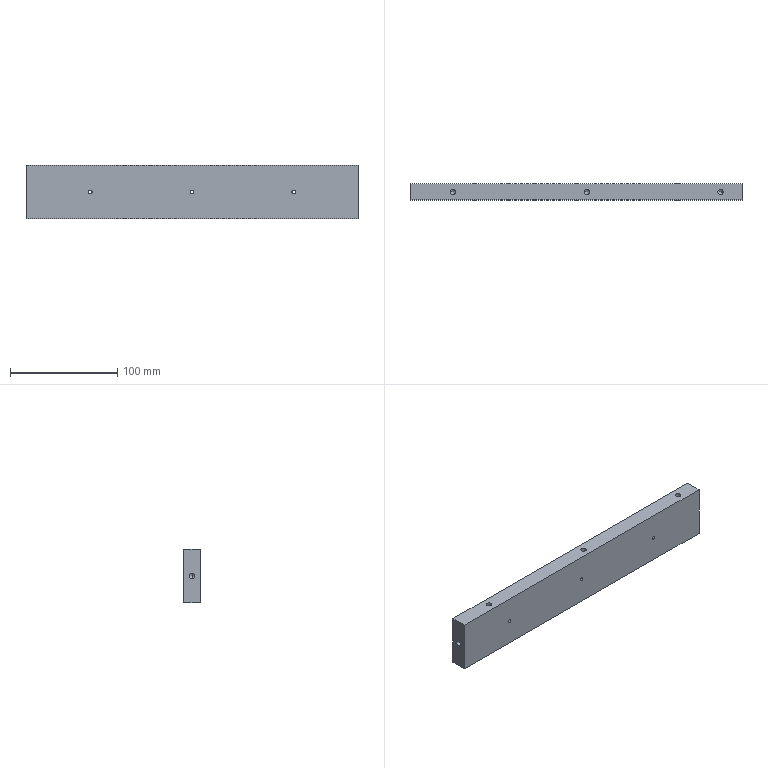Part | SolidWorks | features HoleWzd 4, Extrusion 1 | 1 solid | 32 faces | box 310 x 15 x 50 mm | volume 230397 mm3 | cylinder 16 | cone 10 | plane 6 | commonest cylinder face diameters 5 x10 3.3 x6
STEP:
#1=CARTESIAN_POINT('',(-95.,-7.5,-1.65));
#2=VERTEX_POINT('',#1);
#3=CARTESIAN_POINT('',(-95.,-7.5,1.65));
#4=VERTEX_POINT('',#3);
#5=CARTESIAN_POINT('',(-95.,-7.5,0.));
#6=DIRECTION('',(0.,1.,0.));
#7=DIRECTION('',(0.,0.,1.));
#8=AXIS2_PLACEMENT_3D('',#5,#6,#7);
#9=CIRCLE('',#8,1.65);
#10=EDGE_CURVE('',#2,#4,#9,.T.);
#11=ORIENTED_EDGE('',*,*,#10,.F.);
#12=CARTESIAN_POINT('',(-95.,7.5,-1.65));
#13=VERTEX_POINT('',#12);
#14=CARTESIAN_POINT('',(-95.,7.5,-1.65));
#15=DIRECTION('',(0.,1.,0.));
#16=VECTOR('',#15,1000.);
#17=LINE('',#14,#16);
#18=EDGE_CURVE('',#2,#13,#17,.T.);
#19=ORIENTED_EDGE('',*,*,#18,.T.);
#20=CARTESIAN_POINT('',(-95.,7.5,1.65));
#21=VERTEX_POINT('',#20);
#22=CARTESIAN_POINT('',(-95.,7.5,0.));
#23=DIRECTION('',(0.,1.,0.));
#24=DIRECTION('',(0.,0.,1.));
#25=AXIS2_PLACEMENT_3D('',#22,#23,#24);
#26=CIRCLE('',#25,1.65);
#27=EDGE_CURVE('',#13,#21,#26,.T.);
#28=ORIENTED_EDGE('',*,*,#27,.T.);
#29=CARTESIAN_POINT('',(-95.,7.5,1.65));
#30=DIRECTION('',(0.,1.,0.));
#31=VECTOR('',#30,1000.);
#32=LINE('',#29,#31);
#33=EDGE_CURVE('',#4,#21,#32,.T.);
#34=ORIENTED_EDGE('',*,*,#33,.F.);
#35=EDGE_LOOP('',(#11,#19,#28,#34));
#36=FACE_OUTER_BOUND('',#35,.T.);
#37=CARTESIAN_POINT('',(-95.,7.5,0.));
#38=DIRECTION('',(0.,1.,0.));
#39=DIRECTION('',(0.,0.,1.));
#40=AXIS2_PLACEMENT_3D('',#37,#38,#39);
#41=CYLINDRICAL_SURFACE('',#40,1.65);
#42=ADVANCED_FACE('',(#36),#41,.F.);
#43=CARTESIAN_POINT('',(0.,-7.5,-1.65));
#44=VERTEX_POINT('',#43);
#45=CARTESIAN_POINT('',(0.,-7.5,1.65));
#46=VERTEX_POINT('',#45);
#47=CARTESIAN_POINT('',(0.,-7.5,0.));
#48=DIRECTION('',(0.,1.,0.));
#49=DIRECTION('',(0.,0.,1.));
#50=AXIS2_PLACEMENT_3D('',#47,#48,#49);
#51=CIRCLE('',#50,1.65);
#52=EDGE_CURVE('',#44,#46,#51,.T.);
#53=ORIENTED_EDGE('',*,*,#52,.F.);
#54=CARTESIAN_POINT('',(0.,7.5,-1.65));
#55=VERTEX_POINT('',#54);
#56=CARTESIAN_POINT('',(0.,7.5,-1.65));
#57=DIRECTION('',(0.,1.,0.));
#58=VECTOR('',#57,1000.);
#59=LINE('',#56,#58);
#60=EDGE_CURVE('',#44,#55,#59,.T.);
#61=ORIENTED_EDGE('',*,*,#60,.T.);
#62=CARTESIAN_POINT('',(0.,7.5,1.65));
#63=VERTEX_POINT('',#62);
#64=CARTESIAN_POINT('',(0.,7.5,0.));
#65=DIRECTION('',(0.,1.,0.));
#66=DIRECTION('',(0.,0.,1.));
#67=AXIS2_PLACEMENT_3D('',#64,#65,#66);
#68=CIRCLE('',#67,1.65);
#69=EDGE_CURVE('',#55,#63,#68,.T.);
#70=ORIENTED_EDGE('',*,*,#69,.T.);
#71=CARTESIAN_POINT('',(0.,7.5,1.65));
#72=DIRECTION('',(0.,1.,0.));
#73=VECTOR('',#72,1000.);
#74=LINE('',#71,#73);
#75=EDGE_CURVE('',#46,#63,#74,.T.);
#76=ORIENTED_EDGE('',*,*,#75,.F.);
#77=EDGE_LOOP('',(#53,#61,#70,#76));
#78=FACE_OUTER_BOUND('',#77,.T.);
#79=CARTESIAN_POINT('',(0.,7.5,0.));
#80=DIRECTION('',(0.,1.,0.));
#81=DIRECTION('',(0.,0.,1.));
#82=AXIS2_PLACEMENT_3D('',#79,#80,#81);
#83=CYLINDRICAL_SURFACE('',#82,1.65);
#84=ADVANCED_FACE('',(#78),#83,.F.);
#85=CARTESIAN_POINT('',(95.,-7.5,-1.65));
#86=VERTEX_POINT('',#85);
#87=CARTESIAN_POINT('',(95.,-7.5,1.65));
#88=VERTEX_POINT('',#87);
#89=CARTESIAN_POINT('',(95.,-7.5,0.));
#90=DIRECTION('',(0.,1.,0.));
#91=DIRECTION('',(0.,0.,1.));
#92=AXIS2_PLACEMENT_3D('',#89,#90,#91);
#93=CIRCLE('',#92,1.65);
#94=EDGE_CURVE('',#86,#88,#93,.T.);
#95=ORIENTED_EDGE('',*,*,#94,.F.);
#96=CARTESIAN_POINT('',(95.,7.5,-1.65));
#97=VERTEX_POINT('',#96);
#98=CARTESIAN_POINT('',(95.,7.5,-1.65));
#99=DIRECTION('',(0.,1.,0.));
#100=VECTOR('',#99,1000.);
#101=LINE('',#98,#100);
#102=EDGE_CURVE('',#86,#97,#101,.T.);
#103=ORIENTED_EDGE('',*,*,#102,.T.);
#104=CARTESIAN_POINT('',(95.,7.5,1.65));
#105=VERTEX_POINT('',#104);
#106=CARTESIAN_POINT('',(95.,7.5,0.));
#107=DIRECTION('',(0.,1.,0.));
#108=DIRECTION('',(0.,0.,1.));
#109=AXIS2_PLACEMENT_3D('',#106,#107,#108);
#110=CIRCLE('',#109,1.65);
#111=EDGE_CURVE('',#97,#105,#110,.T.);
#112=ORIENTED_EDGE('',*,*,#111,.T.);
#113=CARTESIAN_POINT('',(95.,7.5,1.65));
#114=DIRECTION('',(0.,1.,0.));
#115=VECTOR('',#114,1000.);
#116=LINE('',#113,#115);
#117=EDGE_CURVE('',#88,#105,#116,.T.);
#118=ORIENTED_EDGE('',*,*,#117,.F.);
#119=EDGE_LOOP('',(#95,#103,#112,#118));
#120=FACE_OUTER_BOUND('',#119,.T.);
#121=CARTESIAN_POINT('',(95.,7.5,0.));
#122=DIRECTION('',(0.,1.,0.));
#123=DIRECTION('',(0.,0.,1.));
#124=AXIS2_PLACEMENT_3D('',#121,#122,#123);
#125=CYLINDRICAL_SURFACE('',#124,1.65);
#126=ADVANCED_FACE('',(#120),#125,.F.);
#127=CARTESIAN_POINT('',(-138.,0.,-2.5));
#128=VERTEX_POINT('',#127);
#129=CARTESIAN_POINT('',(-138.,0.,2.5));
#130=VERTEX_POINT('',#129);
#131=CARTESIAN_POINT('',(-138.,0.,0.));
#132=DIRECTION('',(-1.,0.,0.));
#133=DIRECTION('',(0.,0.,1.));
#134=AXIS2_PLACEMENT_3D('',#131,#132,#133);
#135=CIRCLE('',#134,2.5);
#136=EDGE_CURVE('',#128,#130,#135,.T.);
#137=ORIENTED_EDGE('',*,*,#136,.F.);
#138=CARTESIAN_POINT('',(-155.,0.,-2.5));
#139=VERTEX_POINT('',#138);
#140=CARTESIAN_POINT('',(-155.,0.,-2.5));
#141=DIRECTION('',(-1.,0.,0.));
#142=VECTOR('',#141,1000.);
#143=LINE('',#140,#142);
#144=EDGE_CURVE('',#128,#139,#143,.T.);
#145=ORIENTED_EDGE('',*,*,#144,.T.);
#146=CARTESIAN_POINT('',(-155.,0.,2.5));
#147=VERTEX_POINT('',#146);
#148=CARTESIAN_POINT('',(-155.,0.,0.));
#149=DIRECTION('',(-1.,0.,0.));
#150=DIRECTION('',(0.,0.,1.));
#151=AXIS2_PLACEMENT_3D('',#148,#149,#150);
#152=CIRCLE('',#151,2.5);
#153=EDGE_CURVE('',#139,#147,#152,.T.);
#154=ORIENTED_EDGE('',*,*,#153,.T.);
#155=CARTESIAN_POINT('',(-155.,0.,2.5));
#156=DIRECTION('',(-1.,0.,0.));
#157=VECTOR('',#156,1000.);
#158=LINE('',#155,#157);
#159=EDGE_CURVE('',#130,#147,#158,.T.);
#160=ORIENTED_EDGE('',*,*,#159,.F.);
#161=EDGE_LOOP('',(#137,#145,#154,#160));
#162=FACE_OUTER_BOUND('',#161,.T.);
#163=CARTESIAN_POINT('',(-155.,0.,0.));
#164=DIRECTION('',(-1.,0.,0.));
#165=DIRECTION('',(0.,0.,1.));
#166=AXIS2_PLACEMENT_3D('',#163,#164,#165);
#167=CYLINDRICAL_SURFACE('',#166,2.5);
#168=ADVANCED_FACE('',(#162),#167,.F.);
#169=CARTESIAN_POINT('',(-136.498,0.,0.));
#170=VERTEX_POINT('',#169);
#171=CARTESIAN_POINT('',(-138.,0.,2.5));
#172=DIRECTION('',(-0.515,0.,0.8572));
#173=VECTOR('',#172,1000.);
#174=LINE('',#171,#173);
#175=EDGE_CURVE('',#170,#130,#174,.T.);
#176=ORIENTED_EDGE('',*,*,#175,.F.);
#177=CARTESIAN_POINT('',(-138.,0.,-2.5));
#178=DIRECTION('',(-0.515,0.,-0.8572));
#179=VECTOR('',#178,1000.);
#180=LINE('',#177,#179);
#181=EDGE_CURVE('',#170,#128,#180,.T.);
#182=ORIENTED_EDGE('',*,*,#181,.T.);
#183=ORIENTED_EDGE('',*,*,#136,.T.);
#184=EDGE_LOOP('',(#176,#182,#183));
#185=FACE_OUTER_BOUND('',#184,.T.);
#186=CARTESIAN_POINT('',(-138.,0.,0.));
#187=DIRECTION('',(-1.,0.,0.));
#188=DIRECTION('',(0.,0.,1.));
#189=AXIS2_PLACEMENT_3D('',#186,#187,#188);
#190=CONICAL_SURFACE('',#189,2.5,1.03);
#191=ADVANCED_FACE('',(#185),#190,.F.);
#192=CARTESIAN_POINT('',(138.,0.,2.5));
#193=VERTEX_POINT('',#192);
#194=CARTESIAN_POINT('',(138.,0.,-2.5));
#195=VERTEX_POINT('',#194);
#196=CARTESIAN_POINT('',(138.,0.,0.));
#197=DIRECTION('',(1.,0.,0.));
#198=DIRECTION('',(0.,0.,-1.));
#199=AXIS2_PLACEMENT_3D('',#196,#197,#198);
#200=CIRCLE('',#199,2.5);
#201=EDGE_CURVE('',#193,#195,#200,.T.);
#202=ORIENTED_EDGE('',*,*,#201,.F.);
#203=CARTESIAN_POINT('',(155.,0.,2.5));
#204=VERTEX_POINT('',#203);
#205=CARTESIAN_POINT('',(155.,0.,2.5));
#206=DIRECTION('',(1.,0.,0.));
#207=VECTOR('',#206,1000.);
#208=LINE('',#205,#207);
#209=EDGE_CURVE('',#193,#204,#208,.T.);
#210=ORIENTED_EDGE('',*,*,#209,.T.);
#211=CARTESIAN_POINT('',(155.,0.,-2.5));
#212=VERTEX_POINT('',#211);
#213=CARTESIAN_POINT('',(155.,0.,0.));
#214=DIRECTION('',(1.,0.,0.));
#215=DIRECTION('',(0.,0.,-1.));
#216=AXIS2_PLACEMENT_3D('',#213,#214,#215);
#217=CIRCLE('',#216,2.5);
#218=EDGE_CURVE('',#204,#212,#217,.T.);
#219=ORIENTED_EDGE('',*,*,#218,.T.);
#220=CARTESIAN_POINT('',(155.,0.,-2.5));
#221=DIRECTION('',(1.,0.,0.));
#222=VECTOR('',#221,1000.);
#223=LINE('',#220,#222);
#224=EDGE_CURVE('',#195,#212,#223,.T.);
#225=ORIENTED_EDGE('',*,*,#224,.F.);
#226=EDGE_LOOP('',(#202,#210,#219,#225));
#227=FACE_OUTER_BOUND('',#226,.T.);
#228=CARTESIAN_POINT('',(155.,0.,0.));
#229=DIRECTION('',(1.,0.,0.));
#230=DIRECTION('',(0.,0.,-1.));
#231=AXIS2_PLACEMENT_3D('',#228,#229,#230);
#232=CYLINDRICAL_SURFACE('',#231,2.5);
#233=ADVANCED_FACE('',(#227),#232,.F.);
#234=CARTESIAN_POINT('',(136.498,0.,0.));
#235=VERTEX_POINT('',#234);
#236=CARTESIAN_POINT('',(138.,0.,-2.5));
#237=DIRECTION('',(0.515,0.,-0.8572));
#238=VECTOR('',#237,1000.);
#239=LINE('',#236,#238);
#240=EDGE_CURVE('',#235,#195,#239,.T.);
#241=ORIENTED_EDGE('',*,*,#240,.F.);
#242=CARTESIAN_POINT('',(138.,0.,2.5));
#243=DIRECTION('',(0.515,0.,0.8572));
#244=VECTOR('',#243,1000.);
#245=LINE('',#242,#244);
#246=EDGE_CURVE('',#235,#193,#245,.T.);
#247=ORIENTED_EDGE('',*,*,#246,.T.);
#248=ORIENTED_EDGE('',*,*,#201,.T.);
#249=EDGE_LOOP('',(#241,#247,#248));
#250=FACE_OUTER_BOUND('',#249,.T.);
#251=CARTESIAN_POINT('',(138.,0.,0.));
#252=DIRECTION('',(1.,0.,0.));
#253=DIRECTION('',(0.,0.,-1.));
#254=AXIS2_PLACEMENT_3D('',#251,#252,#253);
#255=CONICAL_SURFACE('',#254,2.5,1.03);
#256=ADVANCED_FACE('',(#250),#255,.F.);
#257=CARTESIAN_POINT('',(-117.5,0.,8.));
#258=VERTEX_POINT('',#257);
#259=CARTESIAN_POINT('',(-112.5,0.,8.));
#260=VERTEX_POINT('',#259);
#261=CARTESIAN_POINT('',(-115.,0.,8.));
#262=DIRECTION('',(0.,0.,1.));
#263=DIRECTION('',(1.,0.,0.));
#264=AXIS2_PLACEMENT_3D('',#261,#262,#263);
#265=CIRCLE('',#264,2.5);
#266=EDGE_CURVE('',#258,#260,#265,.T.);
#267=ORIENTED_EDGE('',*,*,#266,.F.);
#268=CARTESIAN_POINT('',(-117.5,0.,25.));
#269=VERTEX_POINT('',#268);
#270=CARTESIAN_POINT('',(-117.5,0.,25.));
#271=DIRECTION('',(0.,0.,1.));
#272=VECTOR('',#271,1000.);
#273=LINE('',#270,#272);
#274=EDGE_CURVE('',#258,#269,#273,.T.);
#275=ORIENTED_EDGE('',*,*,#274,.T.);
#276=CARTESIAN_POINT('',(-112.5,0.,25.));
#277=VERTEX_POINT('',#276);
#278=CARTESIAN_POINT('',(-115.,0.,25.));
#279=DIRECTION('',(0.,0.,1.));
#280=DIRECTION('',(1.,0.,0.));
#281=AXIS2_PLACEMENT_3D('',#278,#279,#280);
#282=CIRCLE('',#281,2.5);
#283=EDGE_CURVE('',#269,#277,#282,.T.);
#284=ORIENTED_EDGE('',*,*,#283,.T.);
#285=CARTESIAN_POINT('',(-112.5,0.,25.));
#286=DIRECTION('',(0.,0.,1.));
#287=VECTOR('',#286,1000.);
#288=LINE('',#285,#287);
#289=EDGE_CURVE('',#260,#277,#288,.T.);
#290=ORIENTED_EDGE('',*,*,#289,.F.);
#291=EDGE_LOOP('',(#267,#275,#284,#290));
#292=FACE_OUTER_BOUND('',#291,.T.);
#293=CARTESIAN_POINT('',(-115.,0.,25.));
#294=DIRECTION('',(0.,0.,1.));
#295=DIRECTION('',(1.,0.,0.));
#296=AXIS2_PLACEMENT_3D('',#293,#294,#295);
#297=CYLINDRICAL_SURFACE('',#296,2.5);
#298=ADVANCED_FACE('',(#292),#297,.F.);
#299=CARTESIAN_POINT('',(-115.,0.,6.498));
#300=VERTEX_POINT('',#299);
#301=CARTESIAN_POINT('',(-112.5,0.,8.));
#302=DIRECTION('',(0.8572,0.,0.515));
#303=VECTOR('',#302,1000.);
#304=LINE('',#301,#303);
#305=EDGE_CURVE('',#300,#260,#304,.T.);
#306=ORIENTED_EDGE('',*,*,#305,.F.);
#307=CARTESIAN_POINT('',(-117.5,0.,8.));
#308=DIRECTION('',(-0.8572,0.,0.515));
#309=VECTOR('',#308,1000.);
#310=LINE('',#307,#309);
#311=EDGE_CURVE('',#300,#258,#310,.T.);
#312=ORIENTED_EDGE('',*,*,#311,.T.);
#313=ORIENTED_EDGE('',*,*,#266,.T.);
#314=EDGE_LOOP('',(#306,#312,#313));
#315=FACE_OUTER_BOUND('',#314,.T.);
#316=CARTESIAN_POINT('',(-115.,0.,8.));
#317=DIRECTION('',(0.,0.,1.));
#318=DIRECTION('',(1.,0.,0.));
#319=AXIS2_PLACEMENT_3D('',#316,#317,#318);
#320=CONICAL_SURFACE('',#319,2.5,1.03);
#321=ADVANCED_FACE('',(#315),#320,.F.);
#322=CARTESIAN_POINT('',(7.5,0.,8.));
#323=VERTEX_POINT('',#322);
#324=CARTESIAN_POINT('',(12.5,0.,8.));
#325=VERTEX_POINT('',#324);
#326=CARTESIAN_POINT('',(10.,0.,8.));
#327=DIRECTION('',(0.,0.,1.));
#328=DIRECTION('',(1.,0.,0.));
#329=AXIS2_PLACEMENT_3D('',#326,#327,#328);
#330=CIRCLE('',#329,2.5);
#331=EDGE_CURVE('',#323,#325,#330,.T.);
#332=ORIENTED_EDGE('',*,*,#331,.F.);
#333=CARTESIAN_POINT('',(7.5,0.,25.));
#334=VERTEX_POINT('',#333);
#335=CARTESIAN_POINT('',(7.5,0.,25.));
#336=DIRECTION('',(0.,0.,1.));
#337=VECTOR('',#336,1000.);
#338=LINE('',#335,#337);
#339=EDGE_CURVE('',#323,#334,#338,.T.);
#340=ORIENTED_EDGE('',*,*,#339,.T.);
#341=CARTESIAN_POINT('',(12.5,0.,25.));
#342=VERTEX_POINT('',#341);
#343=CARTESIAN_POINT('',(10.,0.,25.));
#344=DIRECTION('',(0.,0.,1.));
#345=DIRECTION('',(1.,0.,0.));
#346=AXIS2_PLACEMENT_3D('',#343,#344,#345);
#347=CIRCLE('',#346,2.5);
#348=EDGE_CURVE('',#334,#342,#347,.T.);
#349=ORIENTED_EDGE('',*,*,#348,.T.);
#350=CARTESIAN_POINT('',(12.5,0.,25.));
#351=DIRECTION('',(0.,0.,1.));
#352=VECTOR('',#351,1000.);
#353=LINE('',#350,#352);
#354=EDGE_CURVE('',#325,#342,#353,.T.);
#355=ORIENTED_EDGE('',*,*,#354,.F.);
#356=EDGE_LOOP('',(#332,#340,#349,#355));
#357=FACE_OUTER_BOUND('',#356,.T.);
#358=CARTESIAN_POINT('',(10.,0.,25.));
#359=DIRECTION('',(0.,0.,1.));
#360=DIRECTION('',(1.,0.,0.));
#361=AXIS2_PLACEMENT_3D('',#358,#359,#360);
#362=CYLINDRICAL_SURFACE('',#361,2.5);
#363=ADVANCED_FACE('',(#357),#362,.F.);
#364=CARTESIAN_POINT('',(10.,0.,6.498));
#365=VERTEX_POINT('',#364);
#366=CARTESIAN_POINT('',(12.5,0.,8.));
#367=DIRECTION('',(0.8572,0.,0.515));
#368=VECTOR('',#367,1000.);
#369=LINE('',#366,#368);
#370=EDGE_CURVE('',#365,#325,#369,.T.);
#371=ORIENTED_EDGE('',*,*,#370,.F.);
#372=CARTESIAN_POINT('',(7.5,0.,8.));
#373=DIRECTION('',(-0.8572,0.,0.515));
#374=VECTOR('',#373,1000.);
#375=LINE('',#372,#374);
#376=EDGE_CURVE('',#365,#323,#375,.T.);
#377=ORIENTED_EDGE('',*,*,#376,.T.);
#378=ORIENTED_EDGE('',*,*,#331,.T.);
#379=EDGE_LOOP('',(#371,#377,#378));
#380=FACE_OUTER_BOUND('',#379,.T.);
#381=CARTESIAN_POINT('',(10.,0.,8.));
#382=DIRECTION('',(0.,0.,1.));
#383=DIRECTION('',(1.,0.,0.));
#384=AXIS2_PLACEMENT_3D('',#381,#382,#383);
#385=CONICAL_SURFACE('',#384,2.5,1.03);
#386=ADVANCED_FACE('',(#380),#385,.F.);
#387=CARTESIAN_POINT('',(132.5,0.,8.));
#388=VERTEX_POINT('',#387);
#389=CARTESIAN_POINT('',(137.5,0.,8.));
#390=VERTEX_POINT('',#389);
#391=CARTESIAN_POINT('',(135.,0.,8.));
#392=DIRECTION('',(0.,0.,1.));
#393=DIRECTION('',(1.,0.,0.));
#394=AXIS2_PLACEMENT_3D('',#391,#392,#393);
#395=CIRCLE('',#394,2.5);
#396=EDGE_CURVE('',#388,#390,#395,.T.);
#397=ORIENTED_EDGE('',*,*,#396,.F.);
#398=CARTESIAN_POINT('',(132.5,0.,25.));
#399=VERTEX_POINT('',#398);
#400=CARTESIAN_POINT('',(132.5,0.,25.));
#401=DIRECTION('',(0.,0.,1.));
#402=VECTOR('',#401,1000.);
#403=LINE('',#400,#402);
#404=EDGE_CURVE('',#388,#399,#403,.T.);
#405=ORIENTED_EDGE('',*,*,#404,.T.);
#406=CARTESIAN_POINT('',(137.5,0.,25.));
#407=VERTEX_POINT('',#406);
#408=CARTESIAN_POINT('',(135.,0.,25.));
#409=DIRECTION('',(0.,0.,1.));
#410=DIRECTION('',(1.,0.,0.));
#411=AXIS2_PLACEMENT_3D('',#408,#409,#410);
#412=CIRCLE('',#411,2.5);
#413=EDGE_CURVE('',#399,#407,#412,.T.);
#414=ORIENTED_EDGE('',*,*,#413,.T.);
#415=CARTESIAN_POINT('',(137.5,0.,25.));
#416=DIRECTION('',(0.,0.,1.));
#417=VECTOR('',#416,1000.);
#418=LINE('',#415,#417);
#419=EDGE_CURVE('',#390,#407,#418,.T.);
#420=ORIENTED_EDGE('',*,*,#419,.F.);
#421=EDGE_LOOP('',(#397,#405,#414,#420));
#422=FACE_OUTER_BOUND('',#421,.T.);
#423=CARTESIAN_POINT('',(135.,0.,25.));
#424=DIRECTION('',(0.,0.,1.));
#425=DIRECTION('',(1.,0.,0.));
#426=AXIS2_PLACEMENT_3D('',#423,#424,#425);
#427=CYLINDRICAL_SURFACE('',#426,2.5);
#428=ADVANCED_FACE('',(#422),#427,.F.);
#429=CARTESIAN_POINT('',(135.,0.,6.498));
#430=VERTEX_POINT('',#429);
#431=CARTESIAN_POINT('',(137.5,0.,8.));
#432=DIRECTION('',(0.8572,0.,0.515));
#433=VECTOR('',#432,1000.);
#434=LINE('',#431,#433);
#435=EDGE_CURVE('',#430,#390,#434,.T.);
#436=ORIENTED_EDGE('',*,*,#435,.F.);
#437=CARTESIAN_POINT('',(132.5,0.,8.));
#438=DIRECTION('',(-0.8572,0.,0.515));
#439=VECTOR('',#438,1000.);
#440=LINE('',#437,#439);
#441=EDGE_CURVE('',#430,#388,#440,.T.);
#442=ORIENTED_EDGE('',*,*,#441,.T.);
#443=ORIENTED_EDGE('',*,*,#396,.T.);
#444=EDGE_LOOP('',(#436,#442,#443));
#445=FACE_OUTER_BOUND('',#444,.T.);
#446=CARTESIAN_POINT('',(135.,0.,8.));
#447=DIRECTION('',(0.,0.,1.));
#448=DIRECTION('',(1.,0.,0.));
#449=AXIS2_PLACEMENT_3D('',#446,#447,#448);
#450=CONICAL_SURFACE('',#449,2.5,1.03);
#451=ADVANCED_FACE('',(#445),#450,.F.);
#452=CARTESIAN_POINT('',(-155.,0.,0.));
#453=DIRECTION('',(-1.,0.,0.));
#454=DIRECTION('',(0.,0.,1.));
#455=AXIS2_PLACEMENT_3D('',#452,#453,#454);
#456=CIRCLE('',#455,2.5);
#457=EDGE_CURVE('',#147,#139,#456,.T.);
#458=ORIENTED_EDGE('',*,*,#457,.F.);
#459=ORIENTED_EDGE('',*,*,#153,.F.);
#460=EDGE_LOOP('',(#458,#459));
#461=FACE_BOUND('',#460,.T.);
#462=CARTESIAN_POINT('',(-155.,-7.5,-25.));
#463=VERTEX_POINT('',#462);
#464=CARTESIAN_POINT('',(-155.,-7.5,25.));
#465=VERTEX_POINT('',#464);
#466=CARTESIAN_POINT('',(-155.,-7.5,25.));
#467=DIRECTION('',(0.,0.,1.));
#468=VECTOR('',#467,1000.);
#469=LINE('',#466,#468);
#470=EDGE_CURVE('',#463,#465,#469,.T.);
#471=ORIENTED_EDGE('',*,*,#470,.T.);
#472=CARTESIAN_POINT('',(-155.,7.5,25.));
#473=VERTEX_POINT('',#472);
#474=CARTESIAN_POINT('',(-155.,7.5,25.));
#475=DIRECTION('',(0.,-1.,0.));
#476=VECTOR('',#475,1000.);
#477=LINE('',#474,#476);
#478=EDGE_CURVE('',#473,#465,#477,.T.);
#479=ORIENTED_EDGE('',*,*,#478,.F.);
#480=CARTESIAN_POINT('',(-155.,7.5,-25.));
#481=VERTEX_POINT('',#480);
#482=CARTESIAN_POINT('',(-155.,7.5,25.));
#483=DIRECTION('',(0.,0.,1.));
#484=VECTOR('',#483,1000.);
#485=LINE('',#482,#484);
#486=EDGE_CURVE('',#481,#473,#485,.T.);
#487=ORIENTED_EDGE('',*,*,#486,.F.);
#488=CARTESIAN_POINT('',(-155.,7.5,-25.));
#489=DIRECTION('',(0.,-1.,0.));
#490=VECTOR('',#489,1000.);
#491=LINE('',#488,#490);
#492=EDGE_CURVE('',#481,#463,#491,.T.);
#493=ORIENTED_EDGE('',*,*,#492,.T.);
#494=EDGE_LOOP('',(#471,#479,#487,#493));
#495=FACE_OUTER_BOUND('',#494,.T.);
#496=CARTESIAN_POINT('',(-155.,7.5,25.));
#497=DIRECTION('',(1.,0.,0.));
#498=DIRECTION('',(0.,0.,-1.));
#499=AXIS2_PLACEMENT_3D('',#496,#497,#498);
#500=PLANE('',#499);
#501=ADVANCED_FACE('',(#461,#495),#500,.F.);
#502=CARTESIAN_POINT('',(-115.,0.,25.));
#503=DIRECTION('',(0.,0.,1.));
#504=DIRECTION('',(1.,0.,0.));
#505=AXIS2_PLACEMENT_3D('',#502,#503,#504);
#506=CIRCLE('',#505,2.5);
#507=EDGE_CURVE('',#277,#269,#506,.T.);
#508=ORIENTED_EDGE('',*,*,#507,.F.);
#509=ORIENTED_EDGE('',*,*,#283,.F.);
#510=EDGE_LOOP('',(#508,#509));
#511=FACE_BOUND('',#510,.T.);
#512=CARTESIAN_POINT('',(10.,0.,25.));
#513=DIRECTION('',(0.,0.,1.));
#514=DIRECTION('',(1.,0.,0.));
#515=AXIS2_PLACEMENT_3D('',#512,#513,#514);
#516=CIRCLE('',#515,2.5);
#517=EDGE_CURVE('',#342,#334,#516,.T.);
#518=ORIENTED_EDGE('',*,*,#517,.F.);
#519=ORIENTED_EDGE('',*,*,#348,.F.);
#520=EDGE_LOOP('',(#518,#519));
#521=FACE_BOUND('',#520,.T.);
#522=CARTESIAN_POINT('',(135.,0.,25.));
#523=DIRECTION('',(0.,0.,1.));
#524=DIRECTION('',(1.,0.,0.));
#525=AXIS2_PLACEMENT_3D('',#522,#523,#524);
#526=CIRCLE('',#525,2.5);
#527=EDGE_CURVE('',#407,#399,#526,.T.);
#528=ORIENTED_EDGE('',*,*,#527,.F.);
#529=ORIENTED_EDGE('',*,*,#413,.F.);
#530=EDGE_LOOP('',(#528,#529));
#531=FACE_BOUND('',#530,.T.);
#532=CARTESIAN_POINT('',(155.,-7.5,25.));
#533=VERTEX_POINT('',#532);
#534=CARTESIAN_POINT('',(155.,-7.5,25.));
#535=DIRECTION('',(1.,0.,0.));
#536=VECTOR('',#535,1000.);
#537=LINE('',#534,#536);
#538=EDGE_CURVE('',#465,#533,#537,.T.);
#539=ORIENTED_EDGE('',*,*,#538,.T.);
#540=CARTESIAN_POINT('',(155.,7.5,25.));
#541=VERTEX_POINT('',#540);
#542=CARTESIAN_POINT('',(155.,7.5,25.));
#543=DIRECTION('',(0.,-1.,0.));
#544=VECTOR('',#543,1000.);
#545=LINE('',#542,#544);
#546=EDGE_CURVE('',#541,#533,#545,.T.);
#547=ORIENTED_EDGE('',*,*,#546,.F.);
#548=CARTESIAN_POINT('',(155.,7.5,25.));
#549=DIRECTION('',(1.,0.,0.));
#550=VECTOR('',#549,1000.);
#551=LINE('',#548,#550);
#552=EDGE_CURVE('',#473,#541,#551,.T.);
#553=ORIENTED_EDGE('',*,*,#552,.F.);
#554=ORIENTED_EDGE('',*,*,#478,.T.);
#555=EDGE_LOOP('',(#539,#547,#553,#554));
#556=FACE_OUTER_BOUND('',#555,.T.);
#557=CARTESIAN_POINT('',(155.,7.5,25.));
#558=DIRECTION('',(0.,0.,-1.));
#559=DIRECTION('',(-1.,0.,0.));
#560=AXIS2_PLACEMENT_3D('',#557,#558,#559);
#561=PLANE('',#560);
#562=ADVANCED_FACE('',(#511,#521,#531,#556),#561,.F.);
#563=CARTESIAN_POINT('',(155.,0.,0.));
#564=DIRECTION('',(1.,0.,0.));
#565=DIRECTION('',(0.,0.,-1.));
#566=AXIS2_PLACEMENT_3D('',#563,#564,#565);
#567=CIRCLE('',#566,2.5);
#568=EDGE_CURVE('',#212,#204,#567,.T.);
#569=ORIENTED_EDGE('',*,*,#568,.F.);
#570=ORIENTED_EDGE('',*,*,#218,.F.);
#571=EDGE_LOOP('',(#569,#570));
#572=FACE_BOUND('',#571,.T.);
#573=CARTESIAN_POINT('',(155.,-7.5,-25.));
#574=VERTEX_POINT('',#573);
#575=CARTESIAN_POINT('',(155.,-7.5,25.));
#576=DIRECTION('',(0.,0.,-1.));
#577=VECTOR('',#576,1000.);
#578=LINE('',#575,#577);
#579=EDGE_CURVE('',#533,#574,#578,.T.);
#580=ORIENTED_EDGE('',*,*,#579,.T.);
#581=CARTESIAN_POINT('',(155.,7.5,-25.));
#582=VERTEX_POINT('',#581);
#583=CARTESIAN_POINT('',(155.,7.5,-25.));
#584=DIRECTION('',(0.,-1.,0.));
#585=VECTOR('',#584,1000.);
#586=LINE('',#583,#585);
#587=EDGE_CURVE('',#582,#574,#586,.T.);
#588=ORIENTED_EDGE('',*,*,#587,.F.);
#589=CARTESIAN_POINT('',(155.,7.5,25.));
#590=DIRECTION('',(0.,0.,-1.));
#591=VECTOR('',#590,1000.);
#592=LINE('',#589,#591);
#593=EDGE_CURVE('',#541,#582,#592,.T.);
#594=ORIENTED_EDGE('',*,*,#593,.F.);
#595=ORIENTED_EDGE('',*,*,#546,.T.);
#596=EDGE_LOOP('',(#580,#588,#594,#595));
#597=FACE_OUTER_BOUND('',#596,.T.);
#598=CARTESIAN_POINT('',(155.,7.5,25.));
#599=DIRECTION('',(-1.,0.,0.));
#600=DIRECTION('',(0.,0.,1.));
#601=AXIS2_PLACEMENT_3D('',#598,#599,#600);
#602=PLANE('',#601);
#603=ADVANCED_FACE('',(#572,#597),#602,.F.);
#604=CARTESIAN_POINT('',(155.,-7.5,-25.));
#605=DIRECTION('',(-1.,0.,0.));
#606=VECTOR('',#605,1000.);
#607=LINE('',#604,#606);
#608=EDGE_CURVE('',#574,#463,#607,.T.);
#609=ORIENTED_EDGE('',*,*,#608,.T.);
#610=ORIENTED_EDGE('',*,*,#492,.F.);
#611=CARTESIAN_POINT('',(155.,7.5,-25.));
#612=DIRECTION('',(-1.,0.,0.));
#613=VECTOR('',#612,1000.);
#614=LINE('',#611,#613);
#615=EDGE_CURVE('',#582,#481,#614,.T.);
#616=ORIENTED_EDGE('',*,*,#615,.F.);
#617=ORIENTED_EDGE('',*,*,#587,.T.);
#618=EDGE_LOOP('',(#609,#610,#616,#617));
#619=FACE_OUTER_BOUND('',#618,.T.);
#620=CARTESIAN_POINT('',(155.,7.5,-25.));
#621=DIRECTION('',(0.,0.,1.));
#622=DIRECTION('',(1.,0.,0.));
#623=AXIS2_PLACEMENT_3D('',#620,#621,#622);
#624=PLANE('',#623);
#625=ADVANCED_FACE('',(#619),#624,.F.);
#626=CARTESIAN_POINT('',(-95.,7.5,0.));
#627=DIRECTION('',(0.,1.,0.));
#628=DIRECTION('',(0.,0.,1.));
#629=AXIS2_PLACEMENT_3D('',#626,#627,#628);
#630=CIRCLE('',#629,1.65);
#631=EDGE_CURVE('',#21,#13,#630,.T.);
#632=ORIENTED_EDGE('',*,*,#631,.F.);
#633=ORIENTED_EDGE('',*,*,#27,.F.);
#634=EDGE_LOOP('',(#632,#633));
#635=FACE_BOUND('',#634,.T.);
#636=CARTESIAN_POINT('',(0.,7.5,0.));
#637=DIRECTION('',(0.,1.,0.));
#638=DIRECTION('',(0.,0.,1.));
#639=AXIS2_PLACEMENT_3D('',#636,#637,#638);
#640=CIRCLE('',#639,1.65);
#641=EDGE_CURVE('',#63,#55,#640,.T.);
#642=ORIENTED_EDGE('',*,*,#641,.F.);
#643=ORIENTED_EDGE('',*,*,#69,.F.);
#644=EDGE_LOOP('',(#642,#643));
#645=FACE_BOUND('',#644,.T.);
#646=CARTESIAN_POINT('',(95.,7.5,0.));
#647=DIRECTION('',(0.,1.,0.));
#648=DIRECTION('',(0.,0.,1.));
#649=AXIS2_PLACEMENT_3D('',#646,#647,#648);
#650=CIRCLE('',#649,1.65);
#651=EDGE_CURVE('',#105,#97,#650,.T.);
#652=ORIENTED_EDGE('',*,*,#651,.F.);
#653=ORIENTED_EDGE('',*,*,#111,.F.);
#654=EDGE_LOOP('',(#652,#653));
#655=FACE_BOUND('',#654,.T.);
#656=ORIENTED_EDGE('',*,*,#486,.T.);
#657=ORIENTED_EDGE('',*,*,#552,.T.);
#658=ORIENTED_EDGE('',*,*,#593,.T.);
#659=ORIENTED_EDGE('',*,*,#615,.T.);
#660=EDGE_LOOP('',(#656,#657,#658,#659));
#661=FACE_OUTER_BOUND('',#660,.T.);
#662=CARTESIAN_POINT('',(0.,7.5,0.));
#663=DIRECTION('',(0.,1.,0.));
#664=DIRECTION('',(0.,0.,1.));
#665=AXIS2_PLACEMENT_3D('',#662,#663,#664);
#666=PLANE('',#665);
#667=ADVANCED_FACE('',(#635,#645,#655,#661),#666,.T.);
#668=CARTESIAN_POINT('',(-95.,-7.5,0.));
#669=DIRECTION('',(0.,1.,0.));
#670=DIRECTION('',(0.,0.,1.));
#671=AXIS2_PLACEMENT_3D('',#668,#669,#670);
#672=CIRCLE('',#671,1.65);
#673=EDGE_CURVE('',#4,#2,#672,.T.);
#674=ORIENTED_EDGE('',*,*,#673,.T.);
#675=ORIENTED_EDGE('',*,*,#10,.T.);
#676=EDGE_LOOP('',(#674,#675));
#677=FACE_BOUND('',#676,.T.);
#678=CARTESIAN_POINT('',(0.,-7.5,0.));
#679=DIRECTION('',(0.,1.,0.));
#680=DIRECTION('',(0.,0.,1.));
#681=AXIS2_PLACEMENT_3D('',#678,#679,#680);
#682=CIRCLE('',#681,1.65);
#683=EDGE_CURVE('',#46,#44,#682,.T.);
#684=ORIENTED_EDGE('',*,*,#683,.T.);
#685=ORIENTED_EDGE('',*,*,#52,.T.);
#686=EDGE_LOOP('',(#684,#685));
#687=FACE_BOUND('',#686,.T.);
#688=CARTESIAN_POINT('',(95.,-7.5,0.));
#689=DIRECTION('',(0.,1.,0.));
#690=DIRECTION('',(0.,0.,1.));
#691=AXIS2_PLACEMENT_3D('',#688,#689,#690);
#692=CIRCLE('',#691,1.65);
#693=EDGE_CURVE('',#88,#86,#692,.T.);
#694=ORIENTED_EDGE('',*,*,#693,.T.);
#695=ORIENTED_EDGE('',*,*,#94,.T.);
#696=EDGE_LOOP('',(#694,#695));
#697=FACE_BOUND('',#696,.T.);
#698=ORIENTED_EDGE('',*,*,#470,.F.);
#699=ORIENTED_EDGE('',*,*,#608,.F.);
#700=ORIENTED_EDGE('',*,*,#579,.F.);
#701=ORIENTED_EDGE('',*,*,#538,.F.);
#702=EDGE_LOOP('',(#698,#699,#700,#701));
#703=FACE_OUTER_BOUND('',#702,.T.);
#704=CARTESIAN_POINT('',(0.,-7.5,0.));
#705=DIRECTION('',(0.,1.,0.));
#706=DIRECTION('',(0.,0.,1.));
#707=AXIS2_PLACEMENT_3D('',#704,#705,#706);
#708=PLANE('',#707);
#709=ADVANCED_FACE('',(#677,#687,#697,#703),#708,.F.);
#710=ORIENTED_EDGE('',*,*,#441,.F.);
#711=ORIENTED_EDGE('',*,*,#435,.T.);
#712=CARTESIAN_POINT('',(135.,0.,8.));
#713=DIRECTION('',(0.,0.,1.));
#714=DIRECTION('',(1.,0.,0.));
#715=AXIS2_PLACEMENT_3D('',#712,#713,#714);
#716=CIRCLE('',#715,2.5);
#717=EDGE_CURVE('',#390,#388,#716,.T.);
#718=ORIENTED_EDGE('',*,*,#717,.T.);
#719=EDGE_LOOP('',(#710,#711,#718));
#720=FACE_OUTER_BOUND('',#719,.T.);
#721=CARTESIAN_POINT('',(135.,0.,8.));
#722=DIRECTION('',(0.,0.,1.));
#723=DIRECTION('',(1.,0.,0.));
#724=AXIS2_PLACEMENT_3D('',#721,#722,#723);
#725=CONICAL_SURFACE('',#724,2.5,1.03);
#726=ADVANCED_FACE('',(#720),#725,.F.);
#727=ORIENTED_EDGE('',*,*,#404,.F.);
#728=ORIENTED_EDGE('',*,*,#717,.F.);
#729=ORIENTED_EDGE('',*,*,#419,.T.);
#730=ORIENTED_EDGE('',*,*,#527,.T.);
#731=EDGE_LOOP('',(#727,#728,#729,#730));
#732=FACE_OUTER_BOUND('',#731,.T.);
#733=CARTESIAN_POINT('',(135.,0.,25.));
#734=DIRECTION('',(0.,0.,1.));
#735=DIRECTION('',(1.,0.,0.));
#736=AXIS2_PLACEMENT_3D('',#733,#734,#735);
#737=CYLINDRICAL_SURFACE('',#736,2.5);
#738=ADVANCED_FACE('',(#732),#737,.F.);
#739=ORIENTED_EDGE('',*,*,#376,.F.);
#740=ORIENTED_EDGE('',*,*,#370,.T.);
#741=CARTESIAN_POINT('',(10.,0.,8.));
#742=DIRECTION('',(0.,0.,1.));
#743=DIRECTION('',(1.,0.,0.));
#744=AXIS2_PLACEMENT_3D('',#741,#742,#743);
#745=CIRCLE('',#744,2.5);
#746=EDGE_CURVE('',#325,#323,#745,.T.);
#747=ORIENTED_EDGE('',*,*,#746,.T.);
#748=EDGE_LOOP('',(#739,#740,#747));
#749=FACE_OUTER_BOUND('',#748,.T.);
#750=CARTESIAN_POINT('',(10.,0.,8.));
#751=DIRECTION('',(0.,0.,1.));
#752=DIRECTION('',(1.,0.,0.));
#753=AXIS2_PLACEMENT_3D('',#750,#751,#752);
#754=CONICAL_SURFACE('',#753,2.5,1.03);
#755=ADVANCED_FACE('',(#749),#754,.F.);
#756=ORIENTED_EDGE('',*,*,#339,.F.);
#757=ORIENTED_EDGE('',*,*,#746,.F.);
#758=ORIENTED_EDGE('',*,*,#354,.T.);
#759=ORIENTED_EDGE('',*,*,#517,.T.);
#760=EDGE_LOOP('',(#756,#757,#758,#759));
#761=FACE_OUTER_BOUND('',#760,.T.);
#762=CARTESIAN_POINT('',(10.,0.,25.));
#763=DIRECTION('',(0.,0.,1.));
#764=DIRECTION('',(1.,0.,0.));
#765=AXIS2_PLACEMENT_3D('',#762,#763,#764);
#766=CYLINDRICAL_SURFACE('',#765,2.5);
#767=ADVANCED_FACE('',(#761),#766,.F.);
#768=ORIENTED_EDGE('',*,*,#311,.F.);
#769=ORIENTED_EDGE('',*,*,#305,.T.);
#770=CARTESIAN_POINT('',(-115.,0.,8.));
#771=DIRECTION('',(0.,0.,1.));
#772=DIRECTION('',(1.,0.,0.));
#773=AXIS2_PLACEMENT_3D('',#770,#771,#772);
#774=CIRCLE('',#773,2.5);
#775=EDGE_CURVE('',#260,#258,#774,.T.);
#776=ORIENTED_EDGE('',*,*,#775,.T.);
#777=EDGE_LOOP('',(#768,#769,#776));
#778=FACE_OUTER_BOUND('',#777,.T.);
#779=CARTESIAN_POINT('',(-115.,0.,8.));
#780=DIRECTION('',(0.,0.,1.));
#781=DIRECTION('',(1.,0.,0.));
#782=AXIS2_PLACEMENT_3D('',#779,#780,#781);
#783=CONICAL_SURFACE('',#782,2.5,1.03);
#784=ADVANCED_FACE('',(#778),#783,.F.);
#785=ORIENTED_EDGE('',*,*,#274,.F.);
#786=ORIENTED_EDGE('',*,*,#775,.F.);
#787=ORIENTED_EDGE('',*,*,#289,.T.);
#788=ORIENTED_EDGE('',*,*,#507,.T.);
#789=EDGE_LOOP('',(#785,#786,#787,#788));
#790=FACE_OUTER_BOUND('',#789,.T.);
#791=CARTESIAN_POINT('',(-115.,0.,25.));
#792=DIRECTION('',(0.,0.,1.));
#793=DIRECTION('',(1.,0.,0.));
#794=AXIS2_PLACEMENT_3D('',#791,#792,#793);
#795=CYLINDRICAL_SURFACE('',#794,2.5);
#796=ADVANCED_FACE('',(#790),#795,.F.);
#797=ORIENTED_EDGE('',*,*,#246,.F.);
#798=ORIENTED_EDGE('',*,*,#240,.T.);
#799=CARTESIAN_POINT('',(138.,0.,0.));
#800=DIRECTION('',(1.,0.,0.));
#801=DIRECTION('',(0.,0.,-1.));
#802=AXIS2_PLACEMENT_3D('',#799,#800,#801);
#803=CIRCLE('',#802,2.5);
#804=EDGE_CURVE('',#195,#193,#803,.T.);
#805=ORIENTED_EDGE('',*,*,#804,.T.);
#806=EDGE_LOOP('',(#797,#798,#805));
#807=FACE_OUTER_BOUND('',#806,.T.);
#808=CARTESIAN_POINT('',(138.,0.,0.));
#809=DIRECTION('',(1.,0.,0.));
#810=DIRECTION('',(0.,0.,-1.));
#811=AXIS2_PLACEMENT_3D('',#808,#809,#810);
#812=CONICAL_SURFACE('',#811,2.5,1.03);
#813=ADVANCED_FACE('',(#807),#812,.F.);
#814=ORIENTED_EDGE('',*,*,#209,.F.);
#815=ORIENTED_EDGE('',*,*,#804,.F.);
#816=ORIENTED_EDGE('',*,*,#224,.T.);
#817=ORIENTED_EDGE('',*,*,#568,.T.);
#818=EDGE_LOOP('',(#814,#815,#816,#817));
#819=FACE_OUTER_BOUND('',#818,.T.);
#820=CARTESIAN_POINT('',(155.,0.,0.));
#821=DIRECTION('',(1.,0.,0.));
#822=DIRECTION('',(0.,0.,-1.));
#823=AXIS2_PLACEMENT_3D('',#820,#821,#822);
#824=CYLINDRICAL_SURFACE('',#823,2.5);
#825=ADVANCED_FACE('',(#819),#824,.F.);
#826=ORIENTED_EDGE('',*,*,#181,.F.);
#827=ORIENTED_EDGE('',*,*,#175,.T.);
#828=CARTESIAN_POINT('',(-138.,0.,0.));
#829=DIRECTION('',(-1.,0.,0.));
#830=DIRECTION('',(0.,0.,1.));
#831=AXIS2_PLACEMENT_3D('',#828,#829,#830);
#832=CIRCLE('',#831,2.5);
#833=EDGE_CURVE('',#130,#128,#832,.T.);
#834=ORIENTED_EDGE('',*,*,#833,.T.);
#835=EDGE_LOOP('',(#826,#827,#834));
#836=FACE_OUTER_BOUND('',#835,.T.);
#837=CARTESIAN_POINT('',(-138.,0.,0.));
#838=DIRECTION('',(-1.,0.,0.));
#839=DIRECTION('',(0.,0.,1.));
#840=AXIS2_PLACEMENT_3D('',#837,#838,#839);
#841=CONICAL_SURFACE('',#840,2.5,1.03);
#842=ADVANCED_FACE('',(#836),#841,.F.);
#843=ORIENTED_EDGE('',*,*,#144,.F.);
#844=ORIENTED_EDGE('',*,*,#833,.F.);
#845=ORIENTED_EDGE('',*,*,#159,.T.);
#846=ORIENTED_EDGE('',*,*,#457,.T.);
#847=EDGE_LOOP('',(#843,#844,#845,#846));
#848=FACE_OUTER_BOUND('',#847,.T.);
#849=CARTESIAN_POINT('',(-155.,0.,0.));
#850=DIRECTION('',(-1.,0.,0.));
#851=DIRECTION('',(0.,0.,1.));
#852=AXIS2_PLACEMENT_3D('',#849,#850,#851);
#853=CYLINDRICAL_SURFACE('',#852,2.5);
#854=ADVANCED_FACE('',(#848),#853,.F.);
#855=ORIENTED_EDGE('',*,*,#102,.F.);
#856=ORIENTED_EDGE('',*,*,#693,.F.);
#857=ORIENTED_EDGE('',*,*,#117,.T.);
#858=ORIENTED_EDGE('',*,*,#651,.T.);
#859=EDGE_LOOP('',(#855,#856,#857,#858));
#860=FACE_OUTER_BOUND('',#859,.T.);
#861=CARTESIAN_POINT('',(95.,7.5,0.));
#862=DIRECTION('',(0.,1.,0.));
#863=DIRECTION('',(0.,0.,1.));
#864=AXIS2_PLACEMENT_3D('',#861,#862,#863);
#865=CYLINDRICAL_SURFACE('',#864,1.65);
#866=ADVANCED_FACE('',(#860),#865,.F.);
#867=ORIENTED_EDGE('',*,*,#60,.F.);
#868=ORIENTED_EDGE('',*,*,#683,.F.);
#869=ORIENTED_EDGE('',*,*,#75,.T.);
#870=ORIENTED_EDGE('',*,*,#641,.T.);
#871=EDGE_LOOP('',(#867,#868,#869,#870));
#872=FACE_OUTER_BOUND('',#871,.T.);
#873=CARTESIAN_POINT('',(0.,7.5,0.));
#874=DIRECTION('',(0.,1.,0.));
#875=DIRECTION('',(0.,0.,1.));
#876=AXIS2_PLACEMENT_3D('',#873,#874,#875);
#877=CYLINDRICAL_SURFACE('',#876,1.65);
#878=ADVANCED_FACE('',(#872),#877,.F.);
#879=ORIENTED_EDGE('',*,*,#18,.F.);
#880=ORIENTED_EDGE('',*,*,#673,.F.);
#881=ORIENTED_EDGE('',*,*,#33,.T.);
#882=ORIENTED_EDGE('',*,*,#631,.T.);
#883=EDGE_LOOP('',(#879,#880,#881,#882));
#884=FACE_OUTER_BOUND('',#883,.T.);
#885=CARTESIAN_POINT('',(-95.,7.5,0.));
#886=DIRECTION('',(0.,1.,0.));
#887=DIRECTION('',(0.,0.,1.));
#888=AXIS2_PLACEMENT_3D('',#885,#886,#887);
#889=CYLINDRICAL_SURFACE('',#888,1.65);
#890=ADVANCED_FACE('',(#884),#889,.F.);
#891=CLOSED_SHELL('',(#42,#84,#126,#168,#191,#233,#256,#298,#321,#363,#386,#428,#451,#501,#562,#603,#625,#667,#709,#726,#738,#755,#767,#784,#796,#813,#825,#842,#854,#866,#878,#890));
#892=MANIFOLD_SOLID_BREP('',#891);
#893=CARTESIAN_POINT('',(0.,0.,0.));
#894=DIRECTION('',(0.,0.,1.));
#895=DIRECTION('',(1.,0.,0.));
#896=AXIS2_PLACEMENT_3D('',#893,#894,#895);
#897=(LENGTH_UNIT()NAMED_UNIT(*)SI_UNIT(.MILLI.,.METRE.));
#898=UNCERTAINTY_MEASURE_WITH_UNIT(LENGTH_MEASURE(0.00001),#897,'','');
#899=(NAMED_UNIT(*)PLANE_ANGLE_UNIT()SI_UNIT($,.RADIAN.));
#900=(NAMED_UNIT(*)SI_UNIT($,.STERADIAN.)SOLID_ANGLE_UNIT());
#901=(GEOMETRIC_REPRESENTATION_CONTEXT(3)GLOBAL_UNCERTAINTY_ASSIGNED_CONTEXT((#898))GLOBAL_UNIT_ASSIGNED_CONTEXT((#897,#899,#900))REPRESENTATION_CONTEXT('',''));
#902=ADVANCED_BREP_SHAPE_REPRESENTATION('',(#892,#896),#901);